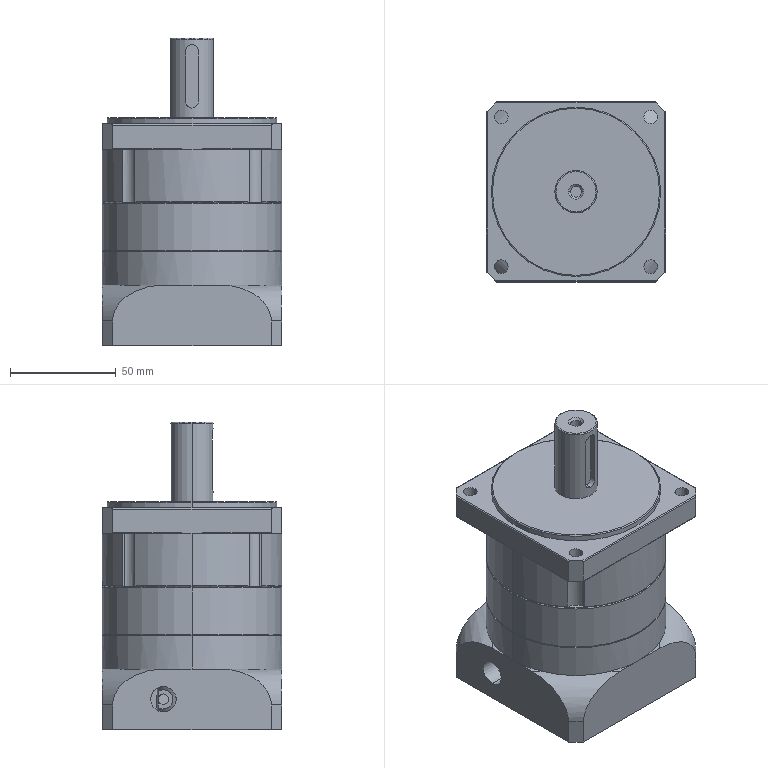Part | SolidWorks | features BaseBody 3 | 3 solids | 160 faces | box 85 x 85 x 145.3 mm | volume 617481 mm3 | cylinder 79 | plane 58 | torus 13 | spline 8 | cone 2 | commonest cylinder face diameters 1 x12 85 x9 4.2 x8 6.5 x8 5 x6 10 x6